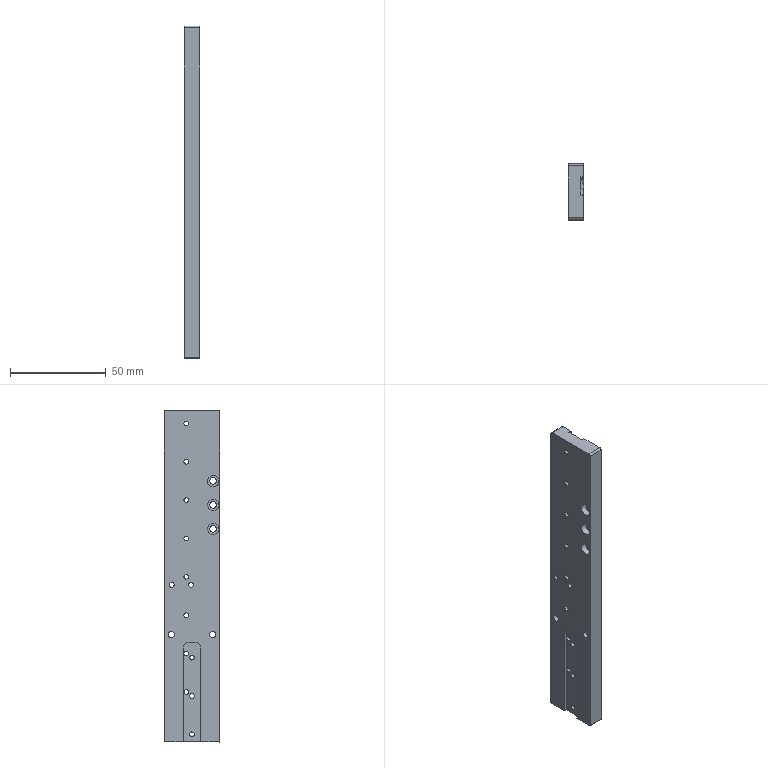CAM job | NX | 3+2 milling, drilling | part box 8 x 29 x 173.1 mm | stock box 10 x 34 x 178.1 mm
Tools:
number,name,description,diameter,corner_radius,flute_length,length,flutes
4,D4,平底铣刀-粗,4.0,0.0,25.0,75.0,2
6,D6,平底铣刀-粗,6.0,0.0,25.0,75.0,2
9,D10,平底铣刀-粗,10.0,0.0,35.0,75.0,2
7,D6-J,平底铣刀-精,6.0,0.0,25.0,75.0,2
10,D10-J,平底铣刀-精,10.0,0.0,35.0,75.0,2
1,D80R0.8_FACEMILL,圆鼻刀-粗,80.0,0.8,50.0,75.0,2
1,D80R0.8_FACEMILL-J,圆鼻刀-精,80.0,0.8,50.0,75.0,2
2,D6_CHAMFER,倒角刀,6.0,0.0,3.0,25.0,2
20,M3X0.5,丝锥,2.5,0.0,35.0,50.0,2
21,M4X0.7,丝锥,3.3,0.0,35.0,50.0,2
12,ZT2.5,钻头,2.5,0.0,35.0,50.0,2
17,ZT3.5,钻头,3.5,0.0,35.0,50.0,2
13,DRILL3.3,Twist Drill 3.3 mm,3.3,0.0,35.0,35.008,2
Operations:
program,operation,operation_type,tool,method,geometry_group,spindle_rpm,surface_speed,feed_per_tooth,feed_cut,feed_plunge,cut_length_mm,path_length_mm,cut_time_min,machine_time_min
B,FLOORWALLMILLFACEMILLONEPASSROUGH_COPY,VolumeBased25DMillingOperation,D80R0.8_FACEMILL,LAYERROUGH-DEPTHK-STEPOVERG,W-B,2800.0,703.696,0.5357,3000.0,100.0,1125.176,1991.434,0.3751,0.4617
B,FLOORWALLMILLFACEMILLONEPASSFINISH_COPY,VolumeBased25DMillingOperation,D80R0.8_FACEMILL-J,SIDEMILLFINISH-DEPTHK-STEPOVERG,W-B,4000.0,1005.28,0.125,1000.0,100.0,281.098,317.098,0.2811,0.2847
B,FLOORWALLROUGH_1_COPY,VolumeBased25DMillingOperation,D6,METHOD,W-B,6000.0,113.0,0.2083,1200.0,100.0,1303.901,1488.926,1.087,1.105
B,DRILLCHAMFER_3,Operation,D6_CHAMFER,METHOD,W-B,8000.0,150.796,0.0625,1000.0,0.0,47.5,334.947,0.0475,0.0762
B,DRILLCHAMFER_4,Operation,D6_CHAMFER,METHOD,W-B,8000.0,150.796,0.0625,1000.0,0.0,10.4,85.508,0.0104,0.0179
B,DRILLCHAMFER_5,Operation,D6_CHAMFER,METHOD,W-B,8000.0,150.796,0.0625,1000.0,0.0,15.15,102.01,0.0151,0.0238
B,PLANARDEBURR6X45L_COPY,SurfaceContour,D6_CHAMFER,SCALLOP_CHAMFER-DEPTH0-STEPOVERG,W-B,6500.0,122.519,0.1154,1500.0,100.0,783.17,1119.62,0.5221,0.5558
B,FLOORSIDEFINISH_3_COPY,VolumeBased25DMillingOperation,D6-J,METHOD,W-B,6000.0,113.0,0.2083,1200.0,100.0,331.232,373.232,0.276,0.2802
A,TOPFACEROUGH,FaceMilling,D80R0.8_FACEMILL,LAYERROUGH-DEPTHK-STEPOVERG,W-A,4000.0,1005.31,0.375,3000.0,100.0,267.1,302.9,0.089,0.0926
A,TOPFACE,FaceMilling,D80R0.8_FACEMILL,SIDEMILLFINISH-DEPTHK-STEPOVERG,W-A,4000.0,1005.31,0.125,1000.0,100.0,267.1,303.1,0.2671,0.2707
A,PROFILEROUGH_2,VolumeBased25DMillingOperation,D10,METHOD,W-A,8000.0,251.327,0.3125,5000.0,80.0,5223.326,5269.926,1.045,1.049
A,SPOTDRILL-DEPTH0.8,Operation,D6_CHAMFER,NONE,W-A,8000.0,150.796,0.0312,500.0,90.0,32.4,367.751,0.0648,0.0983
A,THROUGHHOLE-M3TAPDRILL,Operation,ZT2.5,NONE,W-A,3000.0,23.562,0.05,300.0,90.0,195.0,620.477,0.65,0.6925
A,THROUGHHOLE-M4TAPDRILL,Operation,DRILL3.3,NONE,W-A,3000.0,31.102,0.05,300.0,90.0,29.983,122.489,0.0999,0.1092
A,COUNTERBORE-DRILL0SEG,Operation,ZT3.5,NONE,W-A,2800.0,30.788,0.0179,100.0,90.0,36.154,139.389,0.3615,0.3719
A,DRILLCHAMFER_1,Operation,D6_CHAMFER,METHOD,W-A,8000.0,150.796,0.0312,500.0,0.0,61.75,382.638,0.1235,0.1556
A,DRILLCHAMFER_2,Operation,D6_CHAMFER,METHOD,W-A,8000.0,150.796,0.0312,500.0,0.0,10.4,85.508,0.0208,0.0283
A,THROUGHHOLE-TAPM3,Operation,M3X0.5,METHOD,W-A,800.0,6.283,0.0003,0.5,90.0,139.5,509.477,279.0,279.037
A,THROUGHHOLE-TAPM4,Operation,M4X0.7,METHOD,W-A,600.0,6.22,0.0006,0.7,90.0,24.0,110.523,34.286,34.294
A,FLOORWALLROUGH_1,VolumeBased25DMillingOperation,D6,METHOD,W-A,6000.0,113.0,0.2083,1200.0,100.0,441.926,606.936,0.3683,0.3848
A,HOLEMILLROUGHD4_1,CylinderMilling,D4,NONE,W-A,8000.0,100.531,0.075,1200.0,100.0,223.646,376.146,0.1864,0.2016
A,HOLEMILLFINISHD4_1,CylinderMilling,D4,FINISHSTEPOVERDEPTHOFF,W-A,8000.0,100.531,0.0312,500.0,100.0,44.823,197.323,0.0896,0.1049
A,DRILLCHAMFER_1_COPY,Operation,D6_CHAMFER,METHOD,W-A,8000.0,150.796,0.0312,500.0,0.0,52.25,356.038,0.1045,0.1349
A,SELECTBODYONLY,SurfaceContour,D6_CHAMFER,METHOD,W-A,8000.0,150.796,0.1875,3000.0,100.0,535.075,695.811,0.1784,0.1944
A,MILLCHAMFER_1,PlanarMilling,D6_CHAMFER,NONE,W-A,8000.0,150.796,0.0312,500.0,100.0,83.054,209.464,0.1661,0.1787
A,FLOORSIDEFINISH_3,VolumeBased25DMillingOperation,D6-J,METHOD,W-A,6000.0,113.0,0.2083,1200.0,100.0,110.914,152.914,0.0924,0.0966
A,PROFILESEMIFINISH_2,VolumeBased25DMillingOperation,D10-J,METHOD,W-A,8000.0,251.327,0.0625,1000.0,100.0,439.481,494.681,0.4395,0.445